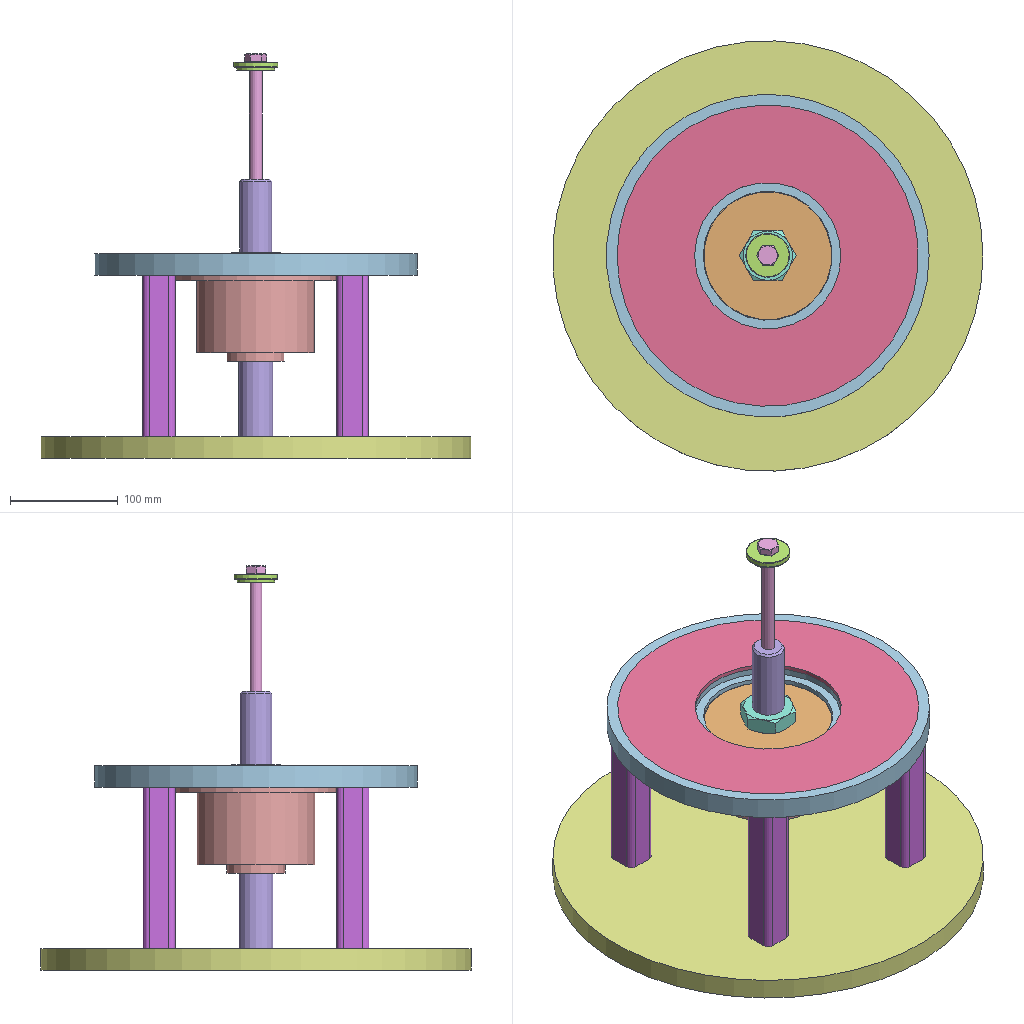Assembly | NX | 11 different items | 17 placed | box 400 x 400 x 376 mm
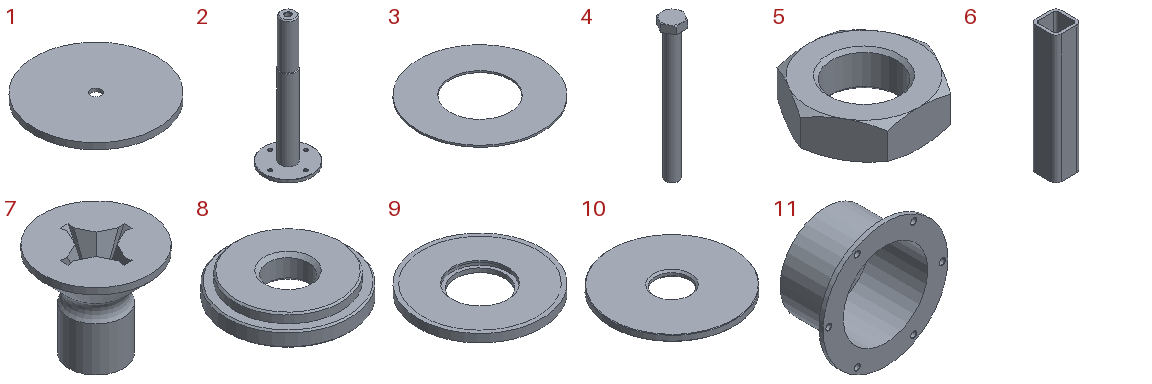Parts list (item | quantity | parent item | size | volume | features):
1 | x1 | - | 400 x 400 x 20 mm | 2431329 mm3 | features HOLE PACKAGE 6, SIMPLE HOLE 6, DATUM_CSYS 5, EXTRACT_DATUM_AXIS 4, EXTRACT_FACE 4, SKETCH 4, SYMBOLIC_THREAD 4, Instance Feature 3, CYLINDER 1, Pattern Feature 1
2 | x1 | - | 95 x 95 x 256 mm | 230884 mm3 | features DATUM_CSYS 5, HOLE PACKAGE 5, CSUNK_HOLE 4, EXTRACT_DATUM_AXIS 4, EXTRACT_FACE 4, SKETCH 4, CHAMFER 3, Instance Feature 3, CYLINDER 2, SYMBOLIC_THREAD 2, EXTRUDE 1, Pattern Feature 1, SIMPLE HOLE 1
3 | x1 | in 9 | 280 x 280 x 4 mm | 188194 mm3 | features BREP 1, DATUM_CSYS 1
4 | x1 | - | 20.785 x 18 x 127.5 mm | 14961 mm3 | features SKETCH 4, EXTRUDE 3, META 3, DATUM_CSYS 2, BLEND 1, CHAMFER 1, LINE 1, SWP104 1, SYMBOLIC_THREAD 1, THREADS 1
5 | x1 | - | 53.116 x 46 x 15 mm | 18421 mm3 | features META 3, SKETCH 3, DATUM_CSYS 2, EXTRUDE 2, SWP104 2, CHAMFER 1, LINE 1, SYMBOLIC_THREAD 1, THREADS 1
6 | x4 | - | 30 x 30 x 150 mm | 45123 mm3 | features DATUM_CSYS 2, EXTRUDE 1, SKETCH 1
7 | x4 | - | 11.3 x 11.3 x 10 mm | 366.572 mm3 | features SKETCH 3, DATUM_CSYS 2, DATUM_PLANE 1, FSET 1, LINE 1, META 1, SKIN 1, SWP104 1, SYMBOLIC_THREAD 1, THREADS 1
8 | x1 | - | 41 x 41 x 8 mm | 8243 mm3 | features CYLINDER 2, CHAMFER 1, DATUM_CSYS 1, HOLE PACKAGE 1, SIMPLE HOLE 1
9 | x1 | - | 300 x 300 x 20 mm | 1155352 mm3 | features HOLE PACKAGE 3, SIMPLE HOLE 3, CYLINDER 1, DATUM_CSYS 1
10 | x1 | - | 120 x 120 x 6 mm | 62323 mm3 | features CHAMFER 1, CYLINDER 1, DATUM_CSYS 1, HOLE PACKAGE 1, SIMPLE HOLE 1
11 | x1 | - | 150 x 80 x 150 mm | 166346 mm3 | features DATUM_CSYS 8, SKETCH 7, EXTRACT_DATUM_AXIS 6, EXTRACT_FACE 6, HOLE PACKAGE 6, SIMPLE HOLE 6, Instance Feature 5, Pattern Feature 1, SWP104 1
Mates (type | each side: item.copy, entity, surface, feature):
Fix | assembly component | 2 times
Bond | 6.1 component | assembly component | 4 times
Linear2dPattern | assembly axis | assembly axis | assembly csys | assembly csys | assembly csys | assembly csys
Distance | 1.1 face cylinder Cylinder(1) | 6.1 face plane Extrude(16) | 2 times
Touch | 9.1 face cylinder Cylinder(1) | 1.1 face cylinder Cylinder(1)
Touch | 1.1 face plane Cylinder(1) | 6.1 face plane Extrude(16)
Fix | 6.1 component
Touch | 9.1 face plane Cylinder(1) | 6.1 face plane Extrude(16)
Touch | 2.1 face cylinder Cylinder(3) | 1.1 face cylinder Ø35 Hole(3)
Touch | 2.1 face plane Cylinder(1) | 1.1 face plane Ø100 Hole(2)
Touch | 5.1 face cylinder Extrude(8) | 2.1 face cylinder Extrude(15)
Touch | 4.1 face plane Extrude(8) | 8.1 face plane Cylinder(1)
Touch | 7.1 face cylinder Revolve(8) | 2.1 face cone M6 Socket Flat Head, 10642 Screw Clearance Hole(5)
Touch | 7.1 face cone Revolve(8) | 2.1 face cone M6 Socket Flat Head, 10642 Screw Clearance Hole(5)
Bond | 2.1 component | assembly component
Bond | 7.1 component | assembly component | 4 times
CircularPattern | assembly axis | assembly csys | assembly csys | assembly csys | assembly csys
Touch | 11.1 face plane Revolve(2) | 9.1 face plane Cylinder(1)
Touch | 10.1 face plane Cylinder(1) | 11.1 face plane Revolve(2)
Touch | 5.1 face plane Extrude(5) | 10.1 face plane Cylinder(1)